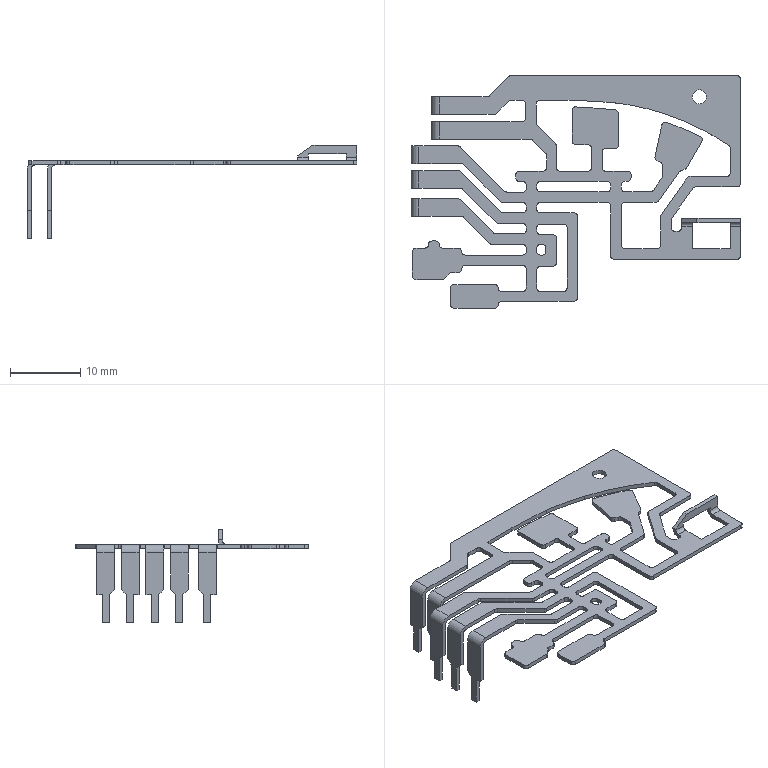Part | NX | features BREP 1 | 1 solid | 293 faces | box 46.9 x 33.1 x 13.3 mm | volume 493.03 mm3 | plane 158 | cylinder 135 | commonest cylinder face diameters 1 x122 2.2 x7 2 x1 69.173 x1 72.496 x1 72.701 x1